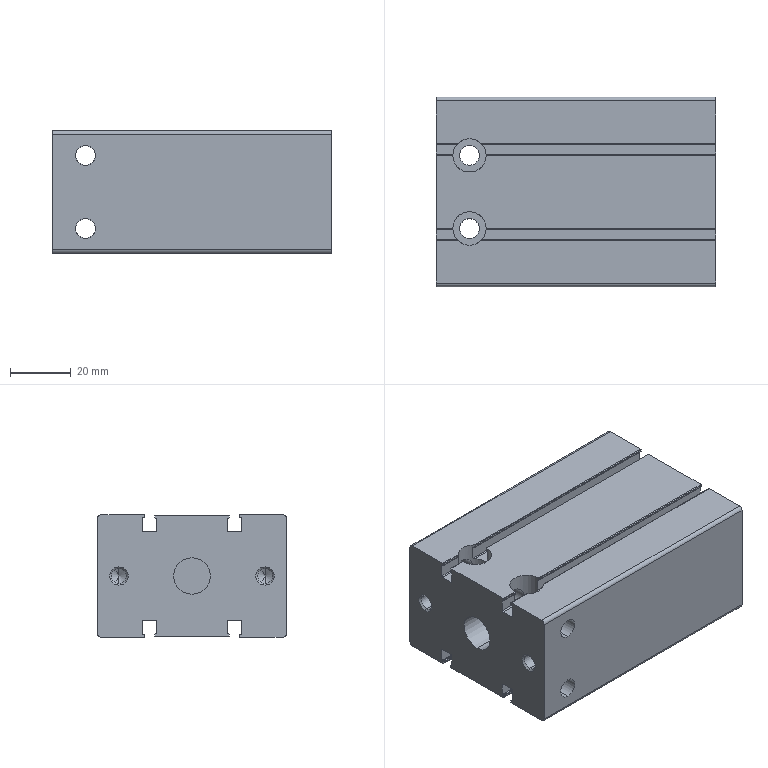Part | STEP file | 11-_MD 32x40-S40 - BodyCW11 | 1 solid | 213 faces | box 92 x 62.3 x 40.3 mm | volume 163773 mm3 | cylinder 118 | plane 75 | cone 20 | commonest cylinder face diameters 0.4 x48 0.8 x16 6.5 x16 11 x16 4.917 x8 2.4 x4